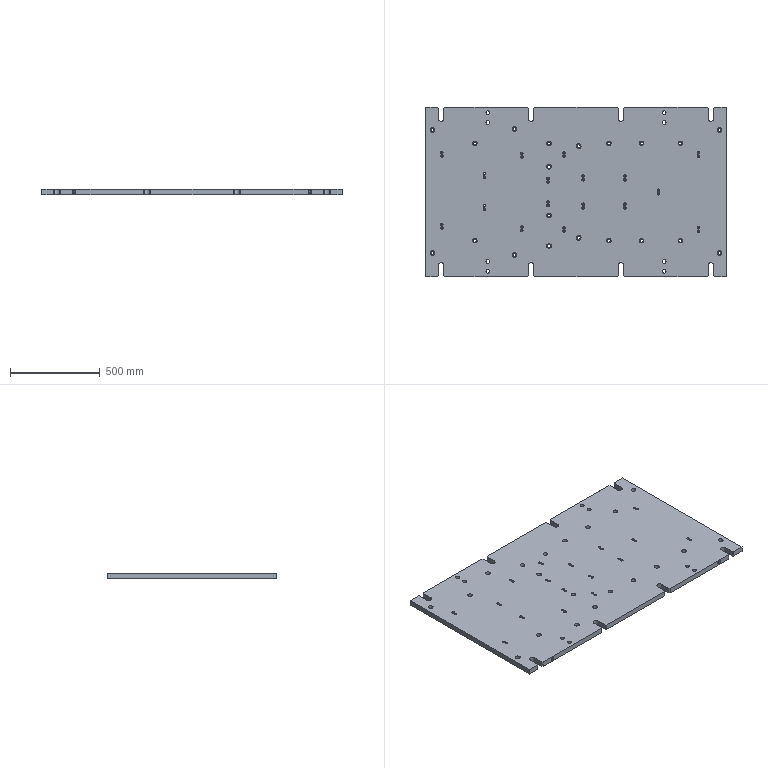Part | NX | features solid 2 | 1 solid | 236 faces | box 1670 x 940 x 30 mm | volume 46056923 mm3 | cylinder 128 | plane 100 | cone 8 | commonest cylinder face diameters 14 x38 9 x34 17 x20 26 x20 21 x8 32 x8